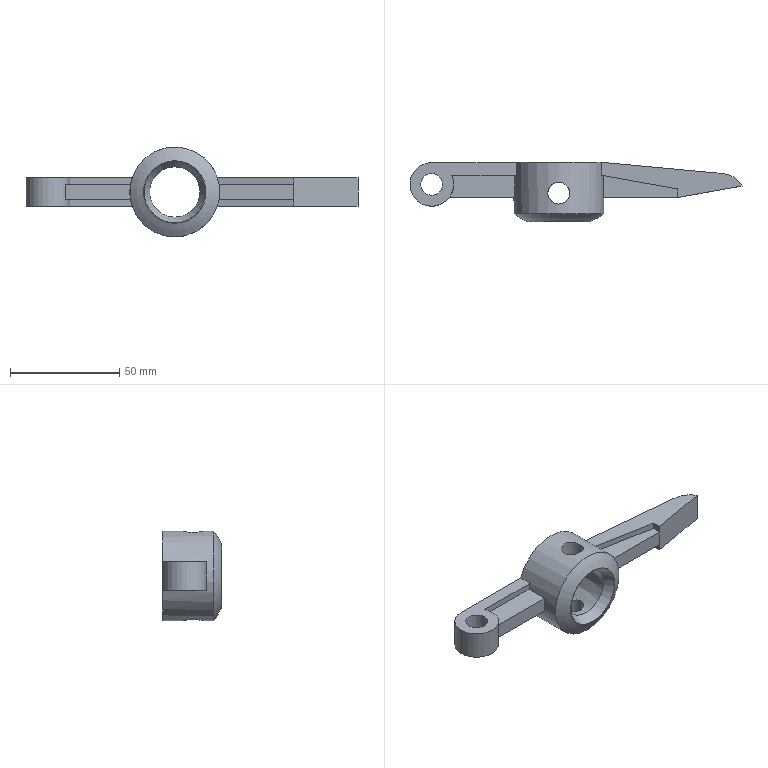Part | NX | features EXTRUDE 7, DATUM_CSYS 5, SKETCH 4, SWP104 3, REPLACE_FACE 2, CHAMFER 1, UNITE 1 | 1 solid | 31 faces | box 151.676 x 27.098 x 41 mm | volume 35006 mm3 | plane 20 | cylinder 8 | cone 2 | sphere 1 | commonest cylinder face diameters 10 x3 41 x3 20 x1 22 x1